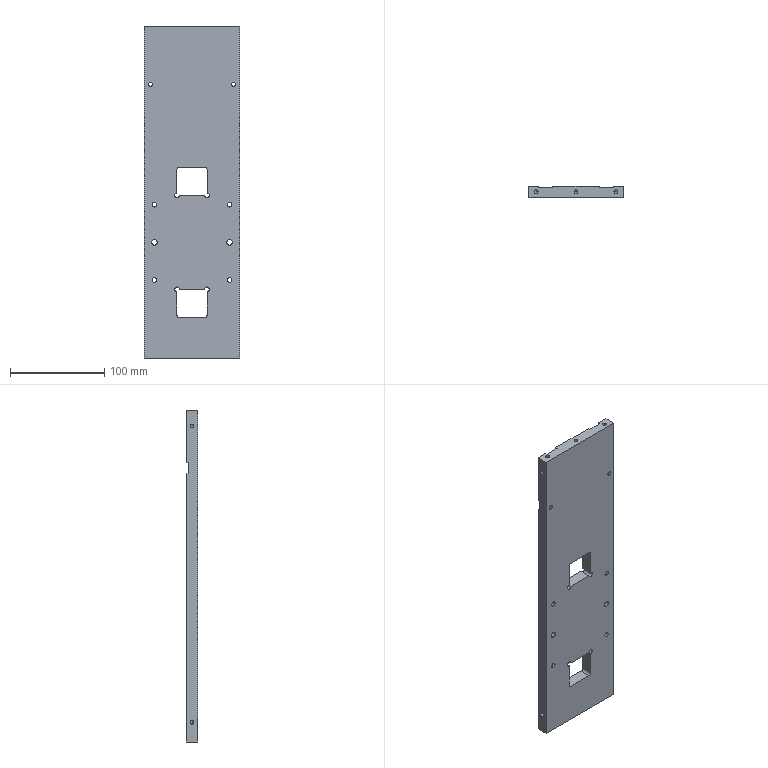Part | SolidWorks | features BaseBody 1 | 1 solid | 162 faces | box 102 x 12 x 353 mm | volume 381378 mm3 | cylinder 74 | cone 48 | plane 40 | commonest cylinder face diameters 2.5 x28 4.2 x24 5 x18 6 x4